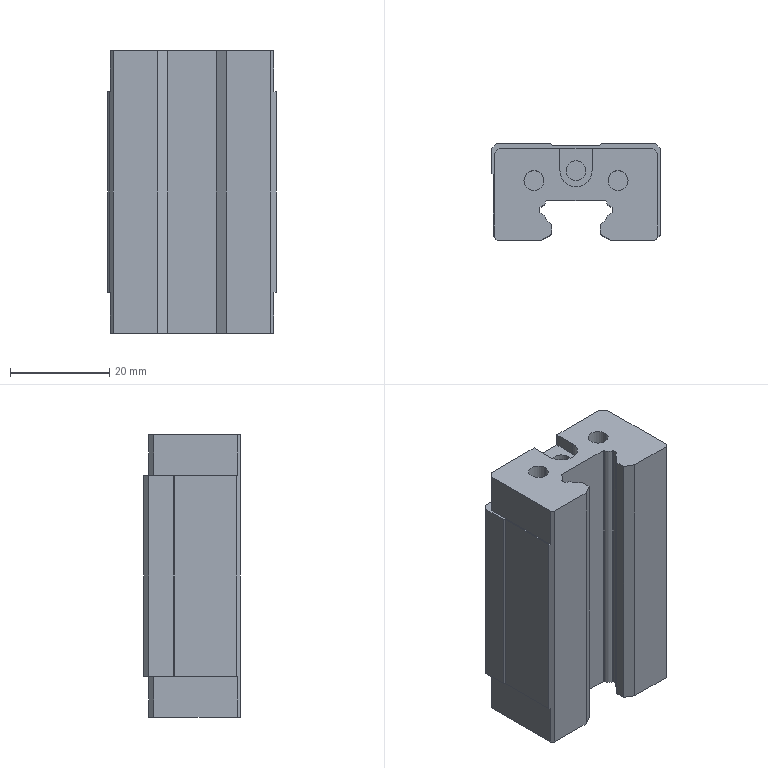Part | STEP file | linear rail slider EGH15CA | 1 solid | 100 faces | box 34 x 19.5 x 57 mm | volume 29973 mm3 | plane 56 | cylinder 28 | cone 16 | commonest cylinder face diameters 4 x12 3.242 x8 3.1 x4 2 x2 6.5 x2